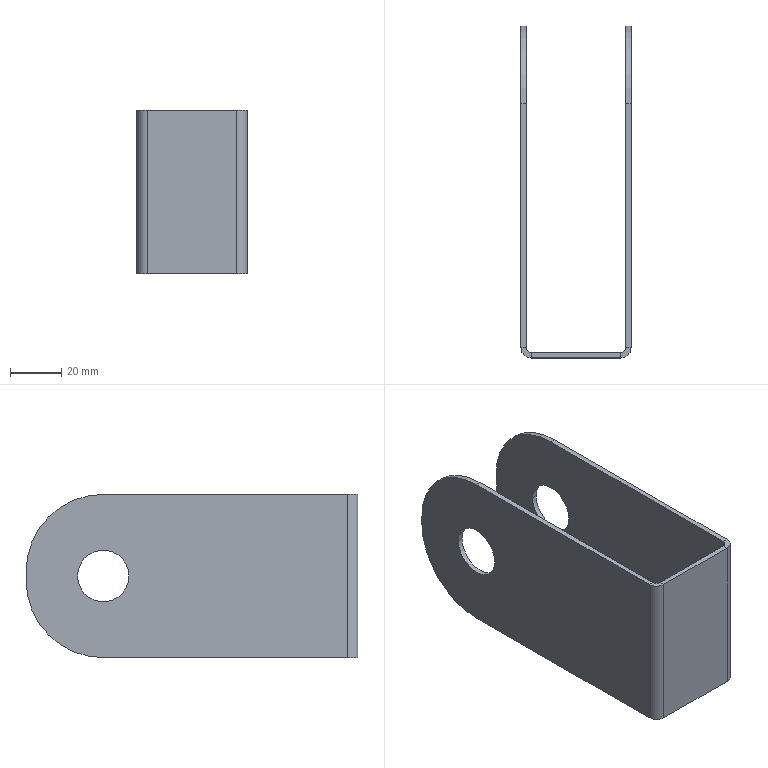Part | SolidWorks | features Fillet 1, FlatPattern 1, ICE 1, SMBaseFlange 1, SheetMetal 1 | 1 solid | 30 faces | box 42.8 x 129 x 63.5 mm | volume 34565 mm3 | plane 18 | cylinder 12 | commonest cylinder face diameters 20 x4 60 x4 4 x2 8 x2
STEP:
#1=CARTESIAN_POINT('',(19.4,107.,31.75));
#2=VERTEX_POINT('',#1);
#3=CARTESIAN_POINT('',(19.4,87.,31.75));
#4=VERTEX_POINT('',#3);
#5=CARTESIAN_POINT('',(19.4,97.,31.75));
#6=DIRECTION('',(-1.,0.,0.));
#7=DIRECTION('',(0.,-1.,0.));
#8=AXIS2_PLACEMENT_3D('',#5,#6,#7);
#9=CIRCLE('',#8,10.);
#10=EDGE_CURVE('',#2,#4,#9,.T.);
#11=ORIENTED_EDGE('',*,*,#10,.T.);
#12=CARTESIAN_POINT('',(21.4,87.,31.75));
#13=VERTEX_POINT('',#12);
#14=CARTESIAN_POINT('',(-49.684,87.,31.75));
#15=DIRECTION('',(1.,0.,0.));
#16=VECTOR('',#15,1000.);
#17=LINE('',#14,#16);
#18=EDGE_CURVE('',#4,#13,#17,.T.);
#19=ORIENTED_EDGE('',*,*,#18,.T.);
#20=CARTESIAN_POINT('',(21.4,107.,31.75));
#21=VERTEX_POINT('',#20);
#22=CARTESIAN_POINT('',(21.4,97.,31.75));
#23=DIRECTION('',(1.,0.,0.));
#24=DIRECTION('',(0.,1.,0.));
#25=AXIS2_PLACEMENT_3D('',#22,#23,#24);
#26=CIRCLE('',#25,10.);
#27=EDGE_CURVE('',#13,#21,#26,.T.);
#28=ORIENTED_EDGE('',*,*,#27,.T.);
#29=CARTESIAN_POINT('',(-49.684,107.,31.75));
#30=DIRECTION('',(1.,0.,0.));
#31=VECTOR('',#30,1000.);
#32=LINE('',#29,#31);
#33=EDGE_CURVE('',#2,#21,#32,.T.);
#34=ORIENTED_EDGE('',*,*,#33,.F.);
#35=EDGE_LOOP('',(#11,#19,#28,#34));
#36=FACE_OUTER_BOUND('',#35,.T.);
#37=CARTESIAN_POINT('',(-49.684,97.,31.75));
#38=DIRECTION('',(1.,0.,0.));
#39=DIRECTION('',(0.,1.,0.));
#40=AXIS2_PLACEMENT_3D('',#37,#38,#39);
#41=CYLINDRICAL_SURFACE('',#40,10.);
#42=ADVANCED_FACE('',(#36),#41,.F.);
#43=CARTESIAN_POINT('',(-21.4,107.,31.75));
#44=VERTEX_POINT('',#43);
#45=CARTESIAN_POINT('',(-21.4,87.,31.75));
#46=VERTEX_POINT('',#45);
#47=CARTESIAN_POINT('',(-21.4,97.,31.75));
#48=DIRECTION('',(-1.,0.,0.));
#49=DIRECTION('',(0.,0.,-1.));
#50=AXIS2_PLACEMENT_3D('',#47,#48,#49);
#51=CIRCLE('',#50,10.);
#52=EDGE_CURVE('',#44,#46,#51,.T.);
#53=ORIENTED_EDGE('',*,*,#52,.T.);
#54=CARTESIAN_POINT('',(-19.4,87.,31.75));
#55=VERTEX_POINT('',#54);
#56=CARTESIAN_POINT('',(-49.684,87.,31.75));
#57=DIRECTION('',(1.,0.,0.));
#58=VECTOR('',#57,1000.);
#59=LINE('',#56,#58);
#60=EDGE_CURVE('',#46,#55,#59,.T.);
#61=ORIENTED_EDGE('',*,*,#60,.T.);
#62=CARTESIAN_POINT('',(-19.4,107.,31.75));
#63=VERTEX_POINT('',#62);
#64=CARTESIAN_POINT('',(-19.4,97.,31.75));
#65=DIRECTION('',(1.,0.,0.));
#66=DIRECTION('',(0.,0.,-1.));
#67=AXIS2_PLACEMENT_3D('',#64,#65,#66);
#68=CIRCLE('',#67,10.);
#69=EDGE_CURVE('',#55,#63,#68,.T.);
#70=ORIENTED_EDGE('',*,*,#69,.T.);
#71=CARTESIAN_POINT('',(-49.684,107.,31.75));
#72=DIRECTION('',(1.,0.,0.));
#73=VECTOR('',#72,1000.);
#74=LINE('',#71,#73);
#75=EDGE_CURVE('',#44,#63,#74,.T.);
#76=ORIENTED_EDGE('',*,*,#75,.F.);
#77=EDGE_LOOP('',(#53,#61,#70,#76));
#78=FACE_OUTER_BOUND('',#77,.T.);
#79=CARTESIAN_POINT('',(-49.684,97.,31.75));
#80=DIRECTION('',(1.,0.,0.));
#81=DIRECTION('',(0.,1.,0.));
#82=AXIS2_PLACEMENT_3D('',#79,#80,#81);
#83=CYLINDRICAL_SURFACE('',#82,10.);
#84=ADVANCED_FACE('',(#78),#83,.F.);
#85=CARTESIAN_POINT('',(-17.4,0.,63.5));
#86=VERTEX_POINT('',#85);
#87=CARTESIAN_POINT('',(-17.4,-2.,63.5));
#88=VERTEX_POINT('',#87);
#89=CARTESIAN_POINT('',(-17.4,0.,63.5));
#90=DIRECTION('',(0.,-1.,0.));
#91=VECTOR('',#90,1000.);
#92=LINE('',#89,#91);
#93=EDGE_CURVE('',#86,#88,#92,.T.);
#94=ORIENTED_EDGE('',*,*,#93,.F.);
#95=CARTESIAN_POINT('',(-19.4,2.,63.5));
#96=VERTEX_POINT('',#95);
#97=CARTESIAN_POINT('',(-17.4,2.,63.5));
#98=DIRECTION('',(0.,0.,1.));
#99=DIRECTION('',(-1.,0.,0.));
#100=AXIS2_PLACEMENT_3D('',#97,#98,#99);
#101=CIRCLE('',#100,2.);
#102=EDGE_CURVE('',#96,#86,#101,.T.);
#103=ORIENTED_EDGE('',*,*,#102,.F.);
#104=CARTESIAN_POINT('',(-21.4,2.,63.5));
#105=VERTEX_POINT('',#104);
#106=CARTESIAN_POINT('',(-21.4,2.,63.5));
#107=DIRECTION('',(1.,0.,0.));
#108=VECTOR('',#107,1000.);
#109=LINE('',#106,#108);
#110=EDGE_CURVE('',#105,#96,#109,.T.);
#111=ORIENTED_EDGE('',*,*,#110,.F.);
#112=CARTESIAN_POINT('',(-17.4,2.,63.5));
#113=DIRECTION('',(0.,0.,1.));
#114=DIRECTION('',(1.,0.,0.));
#115=AXIS2_PLACEMENT_3D('',#112,#113,#114);
#116=CIRCLE('',#115,4.);
#117=EDGE_CURVE('',#105,#88,#116,.T.);
#118=ORIENTED_EDGE('',*,*,#117,.T.);
#119=EDGE_LOOP('',(#94,#103,#111,#118));
#120=FACE_OUTER_BOUND('',#119,.T.);
#121=CARTESIAN_POINT('',(-17.4,0.,63.5));
#122=DIRECTION('',(0.,0.,1.));
#123=DIRECTION('',(1.,0.,0.));
#124=AXIS2_PLACEMENT_3D('',#121,#122,#123);
#125=PLANE('',#124);
#126=ADVANCED_FACE('',(#120),#125,.T.);
#127=CARTESIAN_POINT('',(17.4,0.,63.5));
#128=VERTEX_POINT('',#127);
#129=CARTESIAN_POINT('',(-19.4,0.,63.5));
#130=DIRECTION('',(1.,0.,0.));
#131=VECTOR('',#130,1000.);
#132=LINE('',#129,#131);
#133=EDGE_CURVE('',#86,#128,#132,.T.);
#134=ORIENTED_EDGE('',*,*,#133,.F.);
#135=ORIENTED_EDGE('',*,*,#93,.T.);
#136=CARTESIAN_POINT('',(17.4,-2.,63.5));
#137=VERTEX_POINT('',#136);
#138=CARTESIAN_POINT('',(-19.4,-2.,63.5));
#139=DIRECTION('',(1.,0.,0.));
#140=VECTOR('',#139,1000.);
#141=LINE('',#138,#140);
#142=EDGE_CURVE('',#88,#137,#141,.T.);
#143=ORIENTED_EDGE('',*,*,#142,.T.);
#144=CARTESIAN_POINT('',(17.4,-2.,63.5));
#145=DIRECTION('',(0.,1.,0.));
#146=VECTOR('',#145,1000.);
#147=LINE('',#144,#146);
#148=EDGE_CURVE('',#137,#128,#147,.T.);
#149=ORIENTED_EDGE('',*,*,#148,.T.);
#150=EDGE_LOOP('',(#134,#135,#143,#149));
#151=FACE_OUTER_BOUND('',#150,.T.);
#152=CARTESIAN_POINT('',(-21.4,2.,63.5));
#153=DIRECTION('',(0.,0.,1.));
#154=DIRECTION('',(1.,0.,0.));
#155=AXIS2_PLACEMENT_3D('',#152,#153,#154);
#156=PLANE('',#155);
#157=ADVANCED_FACE('',(#151),#156,.T.);
#158=CARTESIAN_POINT('',(-19.4,2.,0.));
#159=VERTEX_POINT('',#158);
#160=CARTESIAN_POINT('',(-21.4,2.,0.));
#161=VERTEX_POINT('',#160);
#162=CARTESIAN_POINT('',(-19.4,2.,0.));
#163=DIRECTION('',(-1.,0.,0.));
#164=VECTOR('',#163,1000.);
#165=LINE('',#162,#164);
#166=EDGE_CURVE('',#159,#161,#165,.T.);
#167=ORIENTED_EDGE('',*,*,#166,.F.);
#168=CARTESIAN_POINT('',(-17.4,0.,0.));
#169=VERTEX_POINT('',#168);
#170=CARTESIAN_POINT('',(-17.4,2.,0.));
#171=DIRECTION('',(0.,0.,1.));
#172=DIRECTION('',(-1.,0.,0.));
#173=AXIS2_PLACEMENT_3D('',#170,#171,#172);
#174=CIRCLE('',#173,2.);
#175=EDGE_CURVE('',#159,#169,#174,.T.);
#176=ORIENTED_EDGE('',*,*,#175,.T.);
#177=CARTESIAN_POINT('',(-17.4,-2.,0.));
#178=VERTEX_POINT('',#177);
#179=CARTESIAN_POINT('',(-17.4,-2.,0.));
#180=DIRECTION('',(0.,1.,0.));
#181=VECTOR('',#180,1000.);
#182=LINE('',#179,#181);
#183=EDGE_CURVE('',#178,#169,#182,.T.);
#184=ORIENTED_EDGE('',*,*,#183,.F.);
#185=CARTESIAN_POINT('',(-17.4,2.,0.));
#186=DIRECTION('',(0.,0.,1.));
#187=DIRECTION('',(1.,0.,0.));
#188=AXIS2_PLACEMENT_3D('',#185,#186,#187);
#189=CIRCLE('',#188,4.);
#190=EDGE_CURVE('',#161,#178,#189,.T.);
#191=ORIENTED_EDGE('',*,*,#190,.F.);
#192=EDGE_LOOP('',(#167,#176,#184,#191));
#193=FACE_OUTER_BOUND('',#192,.T.);
#194=CARTESIAN_POINT('',(-19.4,2.,0.));
#195=DIRECTION('',(0.,0.,-1.));
#196=DIRECTION('',(-1.,0.,0.));
#197=AXIS2_PLACEMENT_3D('',#194,#195,#196);
#198=PLANE('',#197);
#199=ADVANCED_FACE('',(#193),#198,.T.);
#200=CARTESIAN_POINT('',(-21.4,97.,0.));
#201=VERTEX_POINT('',#200);
#202=CARTESIAN_POINT('',(-21.4,0.,0.));
#203=DIRECTION('',(0.,-1.,0.));
#204=VECTOR('',#203,1000.);
#205=LINE('',#202,#204);
#206=EDGE_CURVE('',#201,#161,#205,.T.);
#207=ORIENTED_EDGE('',*,*,#206,.F.);
#208=CARTESIAN_POINT('',(-19.4,97.,0.));
#209=VERTEX_POINT('',#208);
#210=CARTESIAN_POINT('',(-17.4,97.,0.));
#211=DIRECTION('',(1.,0.,0.));
#212=VECTOR('',#211,1000.);
#213=LINE('',#210,#212);
#214=EDGE_CURVE('',#201,#209,#213,.T.);
#215=ORIENTED_EDGE('',*,*,#214,.T.);
#216=CARTESIAN_POINT('',(-19.4,0.,0.));
#217=DIRECTION('',(0.,-1.,0.));
#218=VECTOR('',#217,1000.);
#219=LINE('',#216,#218);
#220=EDGE_CURVE('',#209,#159,#219,.T.);
#221=ORIENTED_EDGE('',*,*,#220,.T.);
#222=ORIENTED_EDGE('',*,*,#166,.T.);
#223=EDGE_LOOP('',(#207,#215,#221,#222));
#224=FACE_OUTER_BOUND('',#223,.T.);
#225=CARTESIAN_POINT('',(-17.4,-2.,0.));
#226=DIRECTION('',(0.,0.,-1.));
#227=DIRECTION('',(-1.,0.,0.));
#228=AXIS2_PLACEMENT_3D('',#225,#226,#227);
#229=PLANE('',#228);
#230=ADVANCED_FACE('',(#224),#229,.T.);
#231=CARTESIAN_POINT('',(19.4,2.,63.5));
#232=VERTEX_POINT('',#231);
#233=CARTESIAN_POINT('',(21.4,2.,63.5));
#234=VERTEX_POINT('',#233);
#235=CARTESIAN_POINT('',(19.4,2.,63.5));
#236=DIRECTION('',(1.,0.,0.));
#237=VECTOR('',#236,1000.);
#238=LINE('',#235,#237);
#239=EDGE_CURVE('',#232,#234,#238,.T.);
#240=ORIENTED_EDGE('',*,*,#239,.F.);
#241=CARTESIAN_POINT('',(17.4,2.,63.5));
#242=DIRECTION('',(0.,0.,1.));
#243=DIRECTION('',(-1.,0.,0.));
#244=AXIS2_PLACEMENT_3D('',#241,#242,#243);
#245=CIRCLE('',#244,2.);
#246=EDGE_CURVE('',#128,#232,#245,.T.);
#247=ORIENTED_EDGE('',*,*,#246,.F.);
#248=ORIENTED_EDGE('',*,*,#148,.F.);
#249=CARTESIAN_POINT('',(17.4,2.,63.5));
#250=DIRECTION('',(0.,0.,1.));
#251=DIRECTION('',(1.,0.,0.));
#252=AXIS2_PLACEMENT_3D('',#249,#250,#251);
#253=CIRCLE('',#252,4.);
#254=EDGE_CURVE('',#137,#234,#253,.T.);
#255=ORIENTED_EDGE('',*,*,#254,.T.);
#256=EDGE_LOOP('',(#240,#247,#248,#255));
#257=FACE_OUTER_BOUND('',#256,.T.);
#258=CARTESIAN_POINT('',(19.4,2.,63.5));
#259=DIRECTION('',(0.,0.,1.));
#260=DIRECTION('',(1.,0.,0.));
#261=AXIS2_PLACEMENT_3D('',#258,#259,#260);
#262=PLANE('',#261);
#263=ADVANCED_FACE('',(#257),#262,.T.);
#264=CARTESIAN_POINT('',(21.4,97.,63.5));
#265=VERTEX_POINT('',#264);
#266=CARTESIAN_POINT('',(21.4,0.,63.5));
#267=DIRECTION('',(0.,1.,0.));
#268=VECTOR('',#267,1000.);
#269=LINE('',#266,#268);
#270=EDGE_CURVE('',#234,#265,#269,.T.);
#271=ORIENTED_EDGE('',*,*,#270,.T.);
#272=CARTESIAN_POINT('',(19.4,97.,63.5));
#273=VERTEX_POINT('',#272);
#274=CARTESIAN_POINT('',(17.4,97.,63.5));
#275=DIRECTION('',(-1.,0.,0.));
#276=VECTOR('',#275,1000.);
#277=LINE('',#274,#276);
#278=EDGE_CURVE('',#265,#273,#277,.T.);
#279=ORIENTED_EDGE('',*,*,#278,.T.);
#280=CARTESIAN_POINT('',(19.4,0.,63.5));
#281=DIRECTION('',(0.,1.,0.));
#282=VECTOR('',#281,1000.);
#283=LINE('',#280,#282);
#284=EDGE_CURVE('',#232,#273,#283,.T.);
#285=ORIENTED_EDGE('',*,*,#284,.F.);
#286=ORIENTED_EDGE('',*,*,#239,.T.);
#287=EDGE_LOOP('',(#271,#279,#285,#286));
#288=FACE_OUTER_BOUND('',#287,.T.);
#289=CARTESIAN_POINT('',(17.4,-2.,63.5));
#290=DIRECTION('',(0.,0.,1.));
#291=DIRECTION('',(1.,0.,0.));
#292=AXIS2_PLACEMENT_3D('',#289,#290,#291);
#293=PLANE('',#292);
#294=ADVANCED_FACE('',(#288),#293,.T.);
#295=CARTESIAN_POINT('',(17.4,0.,0.));
#296=VERTEX_POINT('',#295);
#297=CARTESIAN_POINT('',(17.4,-2.,0.));
#298=VERTEX_POINT('',#297);
#299=CARTESIAN_POINT('',(17.4,0.,0.));
#300=DIRECTION('',(0.,-1.,0.));
#301=VECTOR('',#300,1000.);
#302=LINE('',#299,#301);
#303=EDGE_CURVE('',#296,#298,#302,.T.);
#304=ORIENTED_EDGE('',*,*,#303,.F.);
#305=CARTESIAN_POINT('',(19.4,2.,0.));
#306=VERTEX_POINT('',#305);
#307=CARTESIAN_POINT('',(17.4,2.,0.));
#308=DIRECTION('',(0.,0.,1.));
#309=DIRECTION('',(-1.,0.,0.));
#310=AXIS2_PLACEMENT_3D('',#307,#308,#309);
#311=CIRCLE('',#310,2.);
#312=EDGE_CURVE('',#296,#306,#311,.T.);
#313=ORIENTED_EDGE('',*,*,#312,.T.);
#314=CARTESIAN_POINT('',(21.4,2.,0.));
#315=VERTEX_POINT('',#314);
#316=CARTESIAN_POINT('',(21.4,2.,0.));
#317=DIRECTION('',(-1.,0.,0.));
#318=VECTOR('',#317,1000.);
#319=LINE('',#316,#318);
#320=EDGE_CURVE('',#315,#306,#319,.T.);
#321=ORIENTED_EDGE('',*,*,#320,.F.);
#322=CARTESIAN_POINT('',(17.4,2.,0.));
#323=DIRECTION('',(0.,0.,1.));
#324=DIRECTION('',(1.,0.,0.));
#325=AXIS2_PLACEMENT_3D('',#322,#323,#324);
#326=CIRCLE('',#325,4.);
#327=EDGE_CURVE('',#298,#315,#326,.T.);
#328=ORIENTED_EDGE('',*,*,#327,.F.);
#329=EDGE_LOOP('',(#304,#313,#321,#328));
#330=FACE_OUTER_BOUND('',#329,.T.);
#331=CARTESIAN_POINT('',(17.4,0.,0.));
#332=DIRECTION('',(0.,0.,-1.));
#333=DIRECTION('',(-1.,0.,0.));
#334=AXIS2_PLACEMENT_3D('',#331,#332,#333);
#335=PLANE('',#334);
#336=ADVANCED_FACE('',(#330),#335,.T.);
#337=CARTESIAN_POINT('',(-19.4,0.,0.));
#338=DIRECTION('',(1.,0.,0.));
#339=VECTOR('',#338,1000.);
#340=LINE('',#337,#339);
#341=EDGE_CURVE('',#169,#296,#340,.T.);
#342=ORIENTED_EDGE('',*,*,#341,.T.);
#343=ORIENTED_EDGE('',*,*,#303,.T.);
#344=CARTESIAN_POINT('',(-19.4,-2.,0.));
#345=DIRECTION('',(1.,0.,0.));
#346=VECTOR('',#345,1000.);
#347=LINE('',#344,#346);
#348=EDGE_CURVE('',#178,#298,#347,.T.);
#349=ORIENTED_EDGE('',*,*,#348,.F.);
#350=ORIENTED_EDGE('',*,*,#183,.T.);
#351=EDGE_LOOP('',(#342,#343,#349,#350));
#352=FACE_OUTER_BOUND('',#351,.T.);
#353=CARTESIAN_POINT('',(21.4,2.,0.));
#354=DIRECTION('',(0.,0.,-1.));
#355=DIRECTION('',(-1.,0.,0.));
#356=AXIS2_PLACEMENT_3D('',#353,#354,#355);
#357=PLANE('',#356);
#358=ADVANCED_FACE('',(#352),#357,.T.);
#359=CARTESIAN_POINT('',(21.4,97.,31.75));
#360=DIRECTION('',(1.,0.,0.));
#361=DIRECTION('',(0.,1.,0.));
#362=AXIS2_PLACEMENT_3D('',#359,#360,#361);
#363=CIRCLE('',#362,10.);
#364=EDGE_CURVE('',#21,#13,#363,.T.);
#365=ORIENTED_EDGE('',*,*,#364,.F.);
#366=ORIENTED_EDGE('',*,*,#27,.F.);
#367=EDGE_LOOP('',(#365,#366));
#368=FACE_BOUND('',#367,.T.);
#369=CARTESIAN_POINT('',(21.4,97.,0.));
#370=VERTEX_POINT('',#369);
#371=CARTESIAN_POINT('',(21.4,0.,0.));
#372=DIRECTION('',(0.,1.,0.));
#373=VECTOR('',#372,1000.);
#374=LINE('',#371,#373);
#375=EDGE_CURVE('',#315,#370,#374,.T.);
#376=ORIENTED_EDGE('',*,*,#375,.T.);
#377=CARTESIAN_POINT('',(21.4,127.,30.));
#378=VERTEX_POINT('',#377);
#379=CARTESIAN_POINT('',(21.4,97.,30.));
#380=DIRECTION('',(1.,0.,0.));
#381=DIRECTION('',(0.,-1.,0.));
#382=AXIS2_PLACEMENT_3D('',#379,#380,#381);
#383=CIRCLE('',#382,30.);
#384=EDGE_CURVE('',#370,#378,#383,.T.);
#385=ORIENTED_EDGE('',*,*,#384,.T.);
#386=CARTESIAN_POINT('',(21.4,127.,33.5));
#387=VERTEX_POINT('',#386);
#388=CARTESIAN_POINT('',(21.4,127.,63.5));
#389=DIRECTION('',(0.,0.,-1.));
#390=VECTOR('',#389,1000.);
#391=LINE('',#388,#390);
#392=EDGE_CURVE('',#387,#378,#391,.T.);
#393=ORIENTED_EDGE('',*,*,#392,.F.);
#394=CARTESIAN_POINT('',(21.4,97.,33.5));
#395=DIRECTION('',(1.,0.,0.));
#396=DIRECTION('',(0.,-1.,0.));
#397=AXIS2_PLACEMENT_3D('',#394,#395,#396);
#398=CIRCLE('',#397,30.);
#399=EDGE_CURVE('',#387,#265,#398,.T.);
#400=ORIENTED_EDGE('',*,*,#399,.T.);
#401=ORIENTED_EDGE('',*,*,#270,.F.);
#402=CARTESIAN_POINT('',(21.4,2.,63.5));
#403=DIRECTION('',(0.,0.,-1.));
#404=VECTOR('',#403,1000.);
#405=LINE('',#402,#404);
#406=EDGE_CURVE('',#234,#315,#405,.T.);
#407=ORIENTED_EDGE('',*,*,#406,.T.);
#408=EDGE_LOOP('',(#376,#385,#393,#400,#401,#407));
#409=FACE_OUTER_BOUND('',#408,.T.);
#410=CARTESIAN_POINT('',(21.4,0.,63.5));
#411=DIRECTION('',(-1.,0.,0.));
#412=DIRECTION('',(0.,-1.,0.));
#413=AXIS2_PLACEMENT_3D('',#410,#411,#412);
#414=PLANE('',#413);
#415=ADVANCED_FACE('',(#368,#409),#414,.F.);
#416=ORIENTED_EDGE('',*,*,#392,.T.);
#417=CARTESIAN_POINT('',(19.4,127.,30.));
#418=VERTEX_POINT('',#417);
#419=CARTESIAN_POINT('',(19.4,127.,30.));
#420=DIRECTION('',(-1.,0.,0.));
#421=VECTOR('',#420,1000.);
#422=LINE('',#419,#421);
#423=EDGE_CURVE('',#378,#418,#422,.T.);
#424=ORIENTED_EDGE('',*,*,#423,.T.);
#425=CARTESIAN_POINT('',(19.4,127.,33.5));
#426=VERTEX_POINT('',#425);
#427=CARTESIAN_POINT('',(19.4,127.,63.5));
#428=DIRECTION('',(0.,0.,-1.));
#429=VECTOR('',#428,1000.);
#430=LINE('',#427,#429);
#431=EDGE_CURVE('',#426,#418,#430,.T.);
#432=ORIENTED_EDGE('',*,*,#431,.F.);
#433=CARTESIAN_POINT('',(19.4,127.,33.5));
#434=DIRECTION('',(1.,0.,0.));
#435=VECTOR('',#434,1000.);
#436=LINE('',#433,#435);
#437=EDGE_CURVE('',#426,#387,#436,.T.);
#438=ORIENTED_EDGE('',*,*,#437,.T.);
#439=EDGE_LOOP('',(#416,#424,#432,#438));
#440=FACE_OUTER_BOUND('',#439,.T.);
#441=CARTESIAN_POINT('',(19.4,127.,63.5));
#442=DIRECTION('',(0.,1.,0.));
#443=DIRECTION('',(0.,0.,1.));
#444=AXIS2_PLACEMENT_3D('',#441,#442,#443);
#445=PLANE('',#444);
#446=ADVANCED_FACE('',(#440),#445,.T.);
#447=ORIENTED_EDGE('',*,*,#10,.F.);
#448=CARTESIAN_POINT('',(19.4,97.,31.75));
#449=DIRECTION('',(-1.,0.,0.));
#450=DIRECTION('',(0.,-1.,0.));
#451=AXIS2_PLACEMENT_3D('',#448,#449,#450);
#452=CIRCLE('',#451,10.);
#453=EDGE_CURVE('',#4,#2,#452,.T.);
#454=ORIENTED_EDGE('',*,*,#453,.F.);
#455=EDGE_LOOP('',(#447,#454));
#456=FACE_BOUND('',#455,.T.);
#457=ORIENTED_EDGE('',*,*,#431,.T.);
#458=CARTESIAN_POINT('',(19.4,97.,0.));
#459=VERTEX_POINT('',#458);
#460=CARTESIAN_POINT('',(19.4,97.,30.));
#461=DIRECTION('',(-1.,0.,0.));
#462=DIRECTION('',(0.,-1.,0.));
#463=AXIS2_PLACEMENT_3D('',#460,#461,#462);
#464=CIRCLE('',#463,30.);
#465=EDGE_CURVE('',#418,#459,#464,.T.);
#466=ORIENTED_EDGE('',*,*,#465,.T.);
#467=CARTESIAN_POINT('',(19.4,0.,0.));
#468=DIRECTION('',(0.,1.,0.));
#469=VECTOR('',#468,1000.);
#470=LINE('',#467,#469);
#471=EDGE_CURVE('',#306,#459,#470,.T.);
#472=ORIENTED_EDGE('',*,*,#471,.F.);
#473=CARTESIAN_POINT('',(19.4,2.,63.5));
#474=DIRECTION('',(0.,0.,-1.));
#475=VECTOR('',#474,1000.);
#476=LINE('',#473,#475);
#477=EDGE_CURVE('',#232,#306,#476,.T.);
#478=ORIENTED_EDGE('',*,*,#477,.F.);
#479=ORIENTED_EDGE('',*,*,#284,.T.);
#480=CARTESIAN_POINT('',(19.4,97.,33.5));
#481=DIRECTION('',(-1.,0.,0.));
#482=DIRECTION('',(0.,-1.,0.));
#483=AXIS2_PLACEMENT_3D('',#480,#481,#482);
#484=CIRCLE('',#483,30.);
#485=EDGE_CURVE('',#273,#426,#484,.T.);
#486=ORIENTED_EDGE('',*,*,#485,.T.);
#487=EDGE_LOOP('',(#457,#466,#472,#478,#479,#486));
#488=FACE_OUTER_BOUND('',#487,.T.);
#489=CARTESIAN_POINT('',(19.4,0.,63.5));
#490=DIRECTION('',(-1.,0.,0.));
#491=DIRECTION('',(0.,-1.,0.));
#492=AXIS2_PLACEMENT_3D('',#489,#490,#491);
#493=PLANE('',#492);
#494=ADVANCED_FACE('',(#456,#488),#493,.T.);
#495=ORIENTED_EDGE('',*,*,#312,.F.);
#496=CARTESIAN_POINT('',(17.4,0.,63.5));
#497=DIRECTION('',(0.,0.,-1.));
#498=VECTOR('',#497,1000.);
#499=LINE('',#496,#498);
#500=EDGE_CURVE('',#128,#296,#499,.T.);
#501=ORIENTED_EDGE('',*,*,#500,.F.);
#502=ORIENTED_EDGE('',*,*,#246,.T.);
#503=ORIENTED_EDGE('',*,*,#477,.T.);
#504=EDGE_LOOP('',(#495,#501,#502,#503));
#505=FACE_OUTER_BOUND('',#504,.T.);
#506=CARTESIAN_POINT('',(17.4,2.,63.5));
#507=DIRECTION('',(0.,0.,-1.));
#508=DIRECTION('',(-1.,0.,0.));
#509=AXIS2_PLACEMENT_3D('',#506,#507,#508);
#510=CYLINDRICAL_SURFACE('',#509,2.);
#511=ADVANCED_FACE('',(#505),#510,.F.);
#512=ORIENTED_EDGE('',*,*,#341,.F.);
#513=CARTESIAN_POINT('',(-17.4,0.,63.5));
#514=DIRECTION('',(0.,0.,-1.));
#515=VECTOR('',#514,1000.);
#516=LINE('',#513,#515);
#517=EDGE_CURVE('',#86,#169,#516,.T.);
#518=ORIENTED_EDGE('',*,*,#517,.F.);
#519=ORIENTED_EDGE('',*,*,#133,.T.);
#520=ORIENTED_EDGE('',*,*,#500,.T.);
#521=EDGE_LOOP('',(#512,#518,#519,#520));
#522=FACE_OUTER_BOUND('',#521,.T.);
#523=CARTESIAN_POINT('',(-19.4,0.,63.5));
#524=DIRECTION('',(0.,1.,0.));
#525=DIRECTION('',(0.,0.,1.));
#526=AXIS2_PLACEMENT_3D('',#523,#524,#525);
#527=PLANE('',#526);
#528=ADVANCED_FACE('',(#522),#527,.T.);
#529=ORIENTED_EDGE('',*,*,#175,.F.);
#530=CARTESIAN_POINT('',(-19.4,2.,63.5));
#531=DIRECTION('',(0.,0.,-1.));
#532=VECTOR('',#531,1000.);
#533=LINE('',#530,#532);
#534=EDGE_CURVE('',#96,#159,#533,.T.);
#535=ORIENTED_EDGE('',*,*,#534,.F.);
#536=ORIENTED_EDGE('',*,*,#102,.T.);
#537=ORIENTED_EDGE('',*,*,#517,.T.);
#538=EDGE_LOOP('',(#529,#535,#536,#537));
#539=FACE_OUTER_BOUND('',#538,.T.);
#540=CARTESIAN_POINT('',(-17.4,2.,63.5));
#541=DIRECTION('',(0.,0.,-1.));
#542=DIRECTION('',(-1.,0.,0.));
#543=AXIS2_PLACEMENT_3D('',#540,#541,#542);
#544=CYLINDRICAL_SURFACE('',#543,2.);
#545=ADVANCED_FACE('',(#539),#544,.F.);
#546=CARTESIAN_POINT('',(-19.4,97.,31.75));
#547=DIRECTION('',(1.,0.,0.));
#548=DIRECTION('',(0.,0.,-1.));
#549=AXIS2_PLACEMENT_3D('',#546,#547,#548);
#550=CIRCLE('',#549,10.);
#551=EDGE_CURVE('',#63,#55,#550,.T.);
#552=ORIENTED_EDGE('',*,*,#551,.F.);
#553=ORIENTED_EDGE('',*,*,#69,.F.);
#554=EDGE_LOOP('',(#552,#553));
#555=FACE_BOUND('',#554,.T.);
#556=CARTESIAN_POINT('',(-19.4,127.,33.5));
#557=VERTEX_POINT('',#556);
#558=CARTESIAN_POINT('',(-19.4,127.,30.));
#559=VERTEX_POINT('',#558);
#560=CARTESIAN_POINT('',(-19.4,127.,63.5));
#561=DIRECTION('',(0.,0.,-1.));
#562=VECTOR('',#561,1000.);
#563=LINE('',#560,#562);
#564=EDGE_CURVE('',#557,#559,#563,.T.);
#565=ORIENTED_EDGE('',*,*,#564,.F.);
#566=CARTESIAN_POINT('',(-19.4,97.,63.5));
#567=VERTEX_POINT('',#566);
#568=CARTESIAN_POINT('',(-19.4,97.,33.5));
#569=DIRECTION('',(1.,0.,0.));
#570=DIRECTION('',(0.,0.,-1.));
#571=AXIS2_PLACEMENT_3D('',#568,#569,#570);
#572=CIRCLE('',#571,30.);
#573=EDGE_CURVE('',#557,#567,#572,.T.);
#574=ORIENTED_EDGE('',*,*,#573,.T.);
#575=CARTESIAN_POINT('',(-19.4,0.,63.5));
#576=DIRECTION('',(0.,-1.,0.));
#577=VECTOR('',#576,1000.);
#578=LINE('',#575,#577);
#579=EDGE_CURVE('',#567,#96,#578,.T.);
#580=ORIENTED_EDGE('',*,*,#579,.T.);
#581=ORIENTED_EDGE('',*,*,#534,.T.);
#582=ORIENTED_EDGE('',*,*,#220,.F.);
#583=CARTESIAN_POINT('',(-19.4,97.,30.));
#584=DIRECTION('',(1.,0.,0.));
#585=DIRECTION('',(0.,0.,-1.));
#586=AXIS2_PLACEMENT_3D('',#583,#584,#585);
#587=CIRCLE('',#586,30.);
#588=EDGE_CURVE('',#209,#559,#587,.T.);
#589=ORIENTED_EDGE('',*,*,#588,.T.);
#590=EDGE_LOOP('',(#565,#574,#580,#581,#582,#589));
#591=FACE_OUTER_BOUND('',#590,.T.);
#592=CARTESIAN_POINT('',(-19.4,0.,63.5));
#593=DIRECTION('',(1.,0.,0.));
#594=DIRECTION('',(0.,0.,-1.));
#595=AXIS2_PLACEMENT_3D('',#592,#593,#594);
#596=PLANE('',#595);
#597=ADVANCED_FACE('',(#555,#591),#596,.T.);
#598=CARTESIAN_POINT('',(-21.4,127.,33.5));
#599=VERTEX_POINT('',#598);
#600=CARTESIAN_POINT('',(-21.4,127.,30.));
#601=VERTEX_POINT('',#600);
#602=CARTESIAN_POINT('',(-21.4,127.,63.5));
#603=DIRECTION('',(0.,0.,-1.));
#604=VECTOR('',#603,1000.);
#605=LINE('',#602,#604);
#606=EDGE_CURVE('',#599,#601,#605,.T.);
#607=ORIENTED_EDGE('',*,*,#606,.F.);
#608=CARTESIAN_POINT('',(-19.4,127.,33.5));
#609=DIRECTION('',(1.,0.,0.));
#610=VECTOR('',#609,1000.);
#611=LINE('',#608,#610);
#612=EDGE_CURVE('',#599,#557,#611,.T.);
#613=ORIENTED_EDGE('',*,*,#612,.T.);
#614=ORIENTED_EDGE('',*,*,#564,.T.);
#615=CARTESIAN_POINT('',(-21.4,127.,30.));
#616=DIRECTION('',(-1.,0.,0.));
#617=VECTOR('',#616,1000.);
#618=LINE('',#615,#617);
#619=EDGE_CURVE('',#559,#601,#618,.T.);
#620=ORIENTED_EDGE('',*,*,#619,.T.);
#621=EDGE_LOOP('',(#607,#613,#614,#620));
#622=FACE_OUTER_BOUND('',#621,.T.);
#623=CARTESIAN_POINT('',(-21.4,127.,63.5));
#624=DIRECTION('',(0.,1.,0.));
#625=DIRECTION('',(0.,0.,1.));
#626=AXIS2_PLACEMENT_3D('',#623,#624,#625);
#627=PLANE('',#626);
#628=ADVANCED_FACE('',(#622),#627,.T.);
#629=ORIENTED_EDGE('',*,*,#52,.F.);
#630=CARTESIAN_POINT('',(-21.4,97.,31.75));
#631=DIRECTION('',(-1.,0.,0.));
#632=DIRECTION('',(0.,0.,-1.));
#633=AXIS2_PLACEMENT_3D('',#630,#631,#632);
#634=CIRCLE('',#633,10.);
#635=EDGE_CURVE('',#46,#44,#634,.T.);
#636=ORIENTED_EDGE('',*,*,#635,.F.);
#637=EDGE_LOOP('',(#629,#636));
#638=FACE_BOUND('',#637,.T.);
#639=CARTESIAN_POINT('',(-21.4,97.,63.5));
#640=VERTEX_POINT('',#639);
#641=CARTESIAN_POINT('',(-21.4,0.,63.5));
#642=DIRECTION('',(0.,-1.,0.));
#643=VECTOR('',#642,1000.);
#644=LINE('',#641,#643);
#645=EDGE_CURVE('',#640,#105,#644,.T.);
#646=ORIENTED_EDGE('',*,*,#645,.F.);
#647=CARTESIAN_POINT('',(-21.4,97.,33.5));
#648=DIRECTION('',(-1.,0.,0.));
#649=DIRECTION('',(0.,0.,-1.));
#650=AXIS2_PLACEMENT_3D('',#647,#648,#649);
#651=CIRCLE('',#650,30.);
#652=EDGE_CURVE('',#640,#599,#651,.T.);
#653=ORIENTED_EDGE('',*,*,#652,.T.);
#654=ORIENTED_EDGE('',*,*,#606,.T.);
#655=CARTESIAN_POINT('',(-21.4,97.,30.));
#656=DIRECTION('',(-1.,0.,0.));
#657=DIRECTION('',(0.,0.,-1.));
#658=AXIS2_PLACEMENT_3D('',#655,#656,#657);
#659=CIRCLE('',#658,30.);
#660=EDGE_CURVE('',#601,#201,#659,.T.);
#661=ORIENTED_EDGE('',*,*,#660,.T.);
#662=ORIENTED_EDGE('',*,*,#206,.T.);
#663=CARTESIAN_POINT('',(-21.4,2.,63.5));
#664=DIRECTION('',(0.,0.,-1.));
#665=VECTOR('',#664,1000.);
#666=LINE('',#663,#665);
#667=EDGE_CURVE('',#105,#161,#666,.T.);
#668=ORIENTED_EDGE('',*,*,#667,.F.);
#669=EDGE_LOOP('',(#646,#653,#654,#661,#662,#668));
#670=FACE_OUTER_BOUND('',#669,.T.);
#671=CARTESIAN_POINT('',(-21.4,0.,63.5));
#672=DIRECTION('',(1.,0.,0.));
#673=DIRECTION('',(0.,0.,-1.));
#674=AXIS2_PLACEMENT_3D('',#671,#672,#673);
#675=PLANE('',#674);
#676=ADVANCED_FACE('',(#638,#670),#675,.F.);
#677=ORIENTED_EDGE('',*,*,#190,.T.);
#678=CARTESIAN_POINT('',(-17.4,-2.,63.5));
#679=DIRECTION('',(0.,0.,-1.));
#680=VECTOR('',#679,1000.);
#681=LINE('',#678,#680);
#682=EDGE_CURVE('',#88,#178,#681,.T.);
#683=ORIENTED_EDGE('',*,*,#682,.F.);
#684=ORIENTED_EDGE('',*,*,#117,.F.);
#685=ORIENTED_EDGE('',*,*,#667,.T.);
#686=EDGE_LOOP('',(#677,#683,#684,#685));
#687=FACE_OUTER_BOUND('',#686,.T.);
#688=CARTESIAN_POINT('',(-17.4,2.,63.5));
#689=DIRECTION('',(0.,0.,-1.));
#690=DIRECTION('',(-1.,0.,0.));
#691=AXIS2_PLACEMENT_3D('',#688,#689,#690);
#692=CYLINDRICAL_SURFACE('',#691,4.);
#693=ADVANCED_FACE('',(#687),#692,.T.);
#694=ORIENTED_EDGE('',*,*,#348,.T.);
#695=CARTESIAN_POINT('',(17.4,-2.,63.5));
#696=DIRECTION('',(0.,0.,-1.));
#697=VECTOR('',#696,1000.);
#698=LINE('',#695,#697);
#699=EDGE_CURVE('',#137,#298,#698,.T.);
#700=ORIENTED_EDGE('',*,*,#699,.F.);
#701=ORIENTED_EDGE('',*,*,#142,.F.);
#702=ORIENTED_EDGE('',*,*,#682,.T.);
#703=EDGE_LOOP('',(#694,#700,#701,#702));
#704=FACE_OUTER_BOUND('',#703,.T.);
#705=CARTESIAN_POINT('',(-19.4,-2.,63.5));
#706=DIRECTION('',(0.,1.,0.));
#707=DIRECTION('',(0.,0.,1.));
#708=AXIS2_PLACEMENT_3D('',#705,#706,#707);
#709=PLANE('',#708);
#710=ADVANCED_FACE('',(#704),#709,.F.);
#711=ORIENTED_EDGE('',*,*,#327,.T.);
#712=ORIENTED_EDGE('',*,*,#406,.F.);
#713=ORIENTED_EDGE('',*,*,#254,.F.);
#714=ORIENTED_EDGE('',*,*,#699,.T.);
#715=EDGE_LOOP('',(#711,#712,#713,#714));
#716=FACE_OUTER_BOUND('',#715,.T.);
#717=CARTESIAN_POINT('',(17.4,2.,63.5));
#718=DIRECTION('',(0.,0.,-1.));
#719=DIRECTION('',(-1.,0.,0.));
#720=AXIS2_PLACEMENT_3D('',#717,#718,#719);
#721=CYLINDRICAL_SURFACE('',#720,4.);
#722=ADVANCED_FACE('',(#716),#721,.T.);
#723=ORIENTED_EDGE('',*,*,#579,.F.);
#724=CARTESIAN_POINT('',(-21.4,97.,63.5));
#725=DIRECTION('',(-1.,0.,0.));
#726=VECTOR('',#725,1000.);
#727=LINE('',#724,#726);
#728=EDGE_CURVE('',#567,#640,#727,.T.);
#729=ORIENTED_EDGE('',*,*,#728,.T.);
#730=ORIENTED_EDGE('',*,*,#645,.T.);
#731=ORIENTED_EDGE('',*,*,#110,.T.);
#732=EDGE_LOOP('',(#723,#729,#730,#731));
#733=FACE_OUTER_BOUND('',#732,.T.);
#734=CARTESIAN_POINT('',(17.4,2.,63.5));
#735=DIRECTION('',(0.,0.,-1.));
#736=DIRECTION('',(-1.,0.,0.));
#737=AXIS2_PLACEMENT_3D('',#734,#735,#736);
#738=PLANE('',#737);
#739=ADVANCED_FACE('',(#733),#738,.F.);
#740=ORIENTED_EDGE('',*,*,#471,.T.);
#741=CARTESIAN_POINT('',(17.4,97.,0.));
#742=DIRECTION('',(1.,0.,0.));
#743=VECTOR('',#742,1000.);
#744=LINE('',#741,#743);
#745=EDGE_CURVE('',#459,#370,#744,.T.);
#746=ORIENTED_EDGE('',*,*,#745,.T.);
#747=ORIENTED_EDGE('',*,*,#375,.F.);
#748=ORIENTED_EDGE('',*,*,#320,.T.);
#749=EDGE_LOOP('',(#740,#746,#747,#748));
#750=FACE_OUTER_BOUND('',#749,.T.);
#751=CARTESIAN_POINT('',(17.4,2.,0.));
#752=DIRECTION('',(0.,0.,-1.));
#753=DIRECTION('',(-1.,0.,0.));
#754=AXIS2_PLACEMENT_3D('',#751,#752,#753);
#755=PLANE('',#754);
#756=ADVANCED_FACE('',(#750),#755,.T.);
#757=ORIENTED_EDGE('',*,*,#652,.F.);
#758=ORIENTED_EDGE('',*,*,#728,.F.);
#759=ORIENTED_EDGE('',*,*,#573,.F.);
#760=ORIENTED_EDGE('',*,*,#612,.F.);
#761=EDGE_LOOP('',(#757,#758,#759,#760));
#762=FACE_OUTER_BOUND('',#761,.T.);
#763=CARTESIAN_POINT('',(-21.4,97.,33.5));
#764=DIRECTION('',(-1.,0.,0.));
#765=DIRECTION('',(0.,0.,1.));
#766=AXIS2_PLACEMENT_3D('',#763,#764,#765);
#767=CYLINDRICAL_SURFACE('',#766,30.);
#768=ADVANCED_FACE('',(#762),#767,.T.);
#769=ORIENTED_EDGE('',*,*,#660,.F.);
#770=ORIENTED_EDGE('',*,*,#619,.F.);
#771=ORIENTED_EDGE('',*,*,#588,.F.);
#772=ORIENTED_EDGE('',*,*,#214,.F.);
#773=EDGE_LOOP('',(#769,#770,#771,#772));
#774=FACE_OUTER_BOUND('',#773,.T.);
#775=CARTESIAN_POINT('',(-17.4,97.,30.));
#776=DIRECTION('',(1.,0.,0.));
#777=DIRECTION('',(0.,0.,-1.));
#778=AXIS2_PLACEMENT_3D('',#775,#776,#777);
#779=CYLINDRICAL_SURFACE('',#778,30.);
#780=ADVANCED_FACE('',(#774),#779,.T.);
#781=ORIENTED_EDGE('',*,*,#465,.F.);
#782=ORIENTED_EDGE('',*,*,#423,.F.);
#783=ORIENTED_EDGE('',*,*,#384,.F.);
#784=ORIENTED_EDGE('',*,*,#745,.F.);
#785=EDGE_LOOP('',(#781,#782,#783,#784));
#786=FACE_OUTER_BOUND('',#785,.T.);
#787=CARTESIAN_POINT('',(17.4,97.,30.));
#788=DIRECTION('',(1.,0.,0.));
#789=DIRECTION('',(0.,0.,-1.));
#790=AXIS2_PLACEMENT_3D('',#787,#788,#789);
#791=CYLINDRICAL_SURFACE('',#790,30.);
#792=ADVANCED_FACE('',(#786),#791,.T.);
#793=ORIENTED_EDGE('',*,*,#485,.F.);
#794=ORIENTED_EDGE('',*,*,#278,.F.);
#795=ORIENTED_EDGE('',*,*,#399,.F.);
#796=ORIENTED_EDGE('',*,*,#437,.F.);
#797=EDGE_LOOP('',(#793,#794,#795,#796));
#798=FACE_OUTER_BOUND('',#797,.T.);
#799=CARTESIAN_POINT('',(19.4,97.,33.5));
#800=DIRECTION('',(1.,0.,0.));
#801=DIRECTION('',(0.,0.,-1.));
#802=AXIS2_PLACEMENT_3D('',#799,#800,#801);
#803=CYLINDRICAL_SURFACE('',#802,30.);
#804=ADVANCED_FACE('',(#798),#803,.T.);
#805=ORIENTED_EDGE('',*,*,#60,.F.);
#806=ORIENTED_EDGE('',*,*,#635,.T.);
#807=ORIENTED_EDGE('',*,*,#75,.T.);
#808=ORIENTED_EDGE('',*,*,#551,.T.);
#809=EDGE_LOOP('',(#805,#806,#807,#808));
#810=FACE_OUTER_BOUND('',#809,.T.);
#811=CARTESIAN_POINT('',(-49.684,97.,31.75));
#812=DIRECTION('',(1.,0.,0.));
#813=DIRECTION('',(0.,1.,0.));
#814=AXIS2_PLACEMENT_3D('',#811,#812,#813);
#815=CYLINDRICAL_SURFACE('',#814,10.);
#816=ADVANCED_FACE('',(#810),#815,.F.);
#817=ORIENTED_EDGE('',*,*,#18,.F.);
#818=ORIENTED_EDGE('',*,*,#453,.T.);
#819=ORIENTED_EDGE('',*,*,#33,.T.);
#820=ORIENTED_EDGE('',*,*,#364,.T.);
#821=EDGE_LOOP('',(#817,#818,#819,#820));
#822=FACE_OUTER_BOUND('',#821,.T.);
#823=CARTESIAN_POINT('',(-49.684,97.,31.75));
#824=DIRECTION('',(1.,0.,0.));
#825=DIRECTION('',(0.,1.,0.));
#826=AXIS2_PLACEMENT_3D('',#823,#824,#825);
#827=CYLINDRICAL_SURFACE('',#826,10.);
#828=ADVANCED_FACE('',(#822),#827,.F.);
#829=CLOSED_SHELL('',(#42,#84,#126,#157,#199,#230,#263,#294,#336,#358,#415,#446,#494,#511,#528,#545,#597,#628,#676,#693,#710,#722,#739,#756,#768,#780,#792,#804,#816,#828));
#830=MANIFOLD_SOLID_BREP('',#829);
#831=CARTESIAN_POINT('',(0.,0.,0.));
#832=DIRECTION('',(0.,0.,1.));
#833=DIRECTION('',(1.,0.,0.));
#834=AXIS2_PLACEMENT_3D('',#831,#832,#833);
#835=(LENGTH_UNIT()NAMED_UNIT(*)SI_UNIT(.MILLI.,.METRE.));
#836=UNCERTAINTY_MEASURE_WITH_UNIT(LENGTH_MEASURE(0.00001),#835,'','');
#837=(NAMED_UNIT(*)PLANE_ANGLE_UNIT()SI_UNIT($,.RADIAN.));
#838=(NAMED_UNIT(*)SI_UNIT($,.STERADIAN.)SOLID_ANGLE_UNIT());
#839=(GEOMETRIC_REPRESENTATION_CONTEXT(3)GLOBAL_UNCERTAINTY_ASSIGNED_CONTEXT((#836))GLOBAL_UNIT_ASSIGNED_CONTEXT((#835,#837,#838))REPRESENTATION_CONTEXT('',''));
#840=ADVANCED_BREP_SHAPE_REPRESENTATION('',(#830,#834),#839);